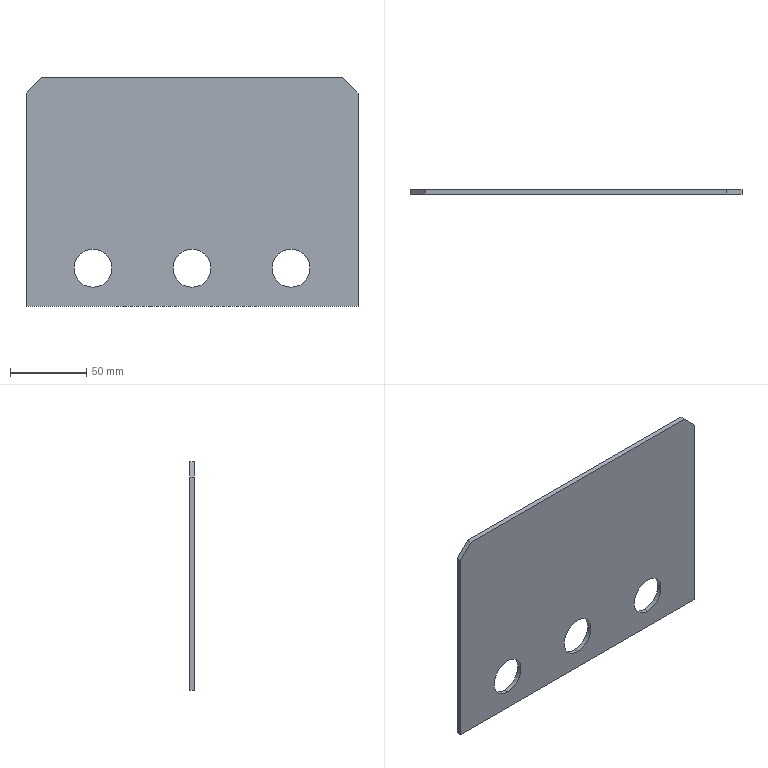Part | SolidWorks | features FlatPattern 1, SMBaseFlange 1, SheetMetal 1 | 1 solid | 14 faces | box 218 x 3 x 150 mm | volume 93382 mm3 | plane 8 | cylinder 6 | commonest cylinder face diameters 25 x6
STEP:
#1=CARTESIAN_POINT('',(65.,3.,-62.5));
#2=VERTEX_POINT('',#1);
#3=CARTESIAN_POINT('',(65.,3.,-37.5));
#4=VERTEX_POINT('',#3);
#5=CARTESIAN_POINT('',(65.,3.,-50.));
#6=DIRECTION('',(0.,1.,0.));
#7=DIRECTION('',(0.,0.,1.));
#8=AXIS2_PLACEMENT_3D('',#5,#6,#7);
#9=CIRCLE('',#8,12.5);
#10=EDGE_CURVE('',#2,#4,#9,.T.);
#11=ORIENTED_EDGE('',*,*,#10,.T.);
#12=CARTESIAN_POINT('',(65.,0.,-37.5));
#13=VERTEX_POINT('',#12);
#14=CARTESIAN_POINT('',(65.,3.,-37.5));
#15=DIRECTION('',(0.,-1.,0.));
#16=VECTOR('',#15,1000.);
#17=LINE('',#14,#16);
#18=EDGE_CURVE('',#4,#13,#17,.T.);
#19=ORIENTED_EDGE('',*,*,#18,.T.);
#20=CARTESIAN_POINT('',(65.,0.,-62.5));
#21=VERTEX_POINT('',#20);
#22=CARTESIAN_POINT('',(65.,0.,-50.));
#23=DIRECTION('',(0.,1.,0.));
#24=DIRECTION('',(0.,0.,1.));
#25=AXIS2_PLACEMENT_3D('',#22,#23,#24);
#26=CIRCLE('',#25,12.5);
#27=EDGE_CURVE('',#21,#13,#26,.T.);
#28=ORIENTED_EDGE('',*,*,#27,.F.);
#29=CARTESIAN_POINT('',(65.,3.,-62.5));
#30=DIRECTION('',(0.,-1.,0.));
#31=VECTOR('',#30,1000.);
#32=LINE('',#29,#31);
#33=EDGE_CURVE('',#2,#21,#32,.T.);
#34=ORIENTED_EDGE('',*,*,#33,.F.);
#35=EDGE_LOOP('',(#11,#19,#28,#34));
#36=FACE_OUTER_BOUND('',#35,.T.);
#37=CARTESIAN_POINT('',(65.,3.,-50.));
#38=DIRECTION('',(0.,-1.,0.));
#39=DIRECTION('',(0.,0.,-1.));
#40=AXIS2_PLACEMENT_3D('',#37,#38,#39);
#41=CYLINDRICAL_SURFACE('',#40,12.5);
#42=ADVANCED_FACE('',(#36),#41,.F.);
#43=CARTESIAN_POINT('',(0.,3.,-62.5));
#44=VERTEX_POINT('',#43);
#45=CARTESIAN_POINT('',(0.,3.,-37.5));
#46=VERTEX_POINT('',#45);
#47=CARTESIAN_POINT('',(0.,3.,-50.));
#48=DIRECTION('',(0.,1.,0.));
#49=DIRECTION('',(0.,0.,1.));
#50=AXIS2_PLACEMENT_3D('',#47,#48,#49);
#51=CIRCLE('',#50,12.5);
#52=EDGE_CURVE('',#44,#46,#51,.T.);
#53=ORIENTED_EDGE('',*,*,#52,.T.);
#54=CARTESIAN_POINT('',(0.,0.,-37.5));
#55=VERTEX_POINT('',#54);
#56=CARTESIAN_POINT('',(0.,3.,-37.5));
#57=DIRECTION('',(0.,-1.,0.));
#58=VECTOR('',#57,1000.);
#59=LINE('',#56,#58);
#60=EDGE_CURVE('',#46,#55,#59,.T.);
#61=ORIENTED_EDGE('',*,*,#60,.T.);
#62=CARTESIAN_POINT('',(0.,0.,-62.5));
#63=VERTEX_POINT('',#62);
#64=CARTESIAN_POINT('',(0.,0.,-50.));
#65=DIRECTION('',(0.,1.,0.));
#66=DIRECTION('',(0.,0.,1.));
#67=AXIS2_PLACEMENT_3D('',#64,#65,#66);
#68=CIRCLE('',#67,12.5);
#69=EDGE_CURVE('',#63,#55,#68,.T.);
#70=ORIENTED_EDGE('',*,*,#69,.F.);
#71=CARTESIAN_POINT('',(0.,3.,-62.5));
#72=DIRECTION('',(0.,-1.,0.));
#73=VECTOR('',#72,1000.);
#74=LINE('',#71,#73);
#75=EDGE_CURVE('',#44,#63,#74,.T.);
#76=ORIENTED_EDGE('',*,*,#75,.F.);
#77=EDGE_LOOP('',(#53,#61,#70,#76));
#78=FACE_OUTER_BOUND('',#77,.T.);
#79=CARTESIAN_POINT('',(0.,3.,-50.));
#80=DIRECTION('',(0.,-1.,0.));
#81=DIRECTION('',(0.,0.,-1.));
#82=AXIS2_PLACEMENT_3D('',#79,#80,#81);
#83=CYLINDRICAL_SURFACE('',#82,12.5);
#84=ADVANCED_FACE('',(#78),#83,.F.);
#85=CARTESIAN_POINT('',(-65.,3.,-62.5));
#86=VERTEX_POINT('',#85);
#87=CARTESIAN_POINT('',(-65.,3.,-37.5));
#88=VERTEX_POINT('',#87);
#89=CARTESIAN_POINT('',(-65.,3.,-50.));
#90=DIRECTION('',(0.,1.,0.));
#91=DIRECTION('',(0.,0.,1.));
#92=AXIS2_PLACEMENT_3D('',#89,#90,#91);
#93=CIRCLE('',#92,12.5);
#94=EDGE_CURVE('',#86,#88,#93,.T.);
#95=ORIENTED_EDGE('',*,*,#94,.T.);
#96=CARTESIAN_POINT('',(-65.,0.,-37.5));
#97=VERTEX_POINT('',#96);
#98=CARTESIAN_POINT('',(-65.,3.,-37.5));
#99=DIRECTION('',(0.,-1.,0.));
#100=VECTOR('',#99,1000.);
#101=LINE('',#98,#100);
#102=EDGE_CURVE('',#88,#97,#101,.T.);
#103=ORIENTED_EDGE('',*,*,#102,.T.);
#104=CARTESIAN_POINT('',(-65.,0.,-62.5));
#105=VERTEX_POINT('',#104);
#106=CARTESIAN_POINT('',(-65.,0.,-50.));
#107=DIRECTION('',(0.,1.,0.));
#108=DIRECTION('',(0.,0.,1.));
#109=AXIS2_PLACEMENT_3D('',#106,#107,#108);
#110=CIRCLE('',#109,12.5);
#111=EDGE_CURVE('',#105,#97,#110,.T.);
#112=ORIENTED_EDGE('',*,*,#111,.F.);
#113=CARTESIAN_POINT('',(-65.,3.,-62.5));
#114=DIRECTION('',(0.,-1.,0.));
#115=VECTOR('',#114,1000.);
#116=LINE('',#113,#115);
#117=EDGE_CURVE('',#86,#105,#116,.T.);
#118=ORIENTED_EDGE('',*,*,#117,.F.);
#119=EDGE_LOOP('',(#95,#103,#112,#118));
#120=FACE_OUTER_BOUND('',#119,.T.);
#121=CARTESIAN_POINT('',(-65.,3.,-50.));
#122=DIRECTION('',(0.,-1.,0.));
#123=DIRECTION('',(0.,0.,-1.));
#124=AXIS2_PLACEMENT_3D('',#121,#122,#123);
#125=CYLINDRICAL_SURFACE('',#124,12.5);
#126=ADVANCED_FACE('',(#120),#125,.F.);
#127=ORIENTED_EDGE('',*,*,#52,.F.);
#128=CARTESIAN_POINT('',(0.,3.,-50.));
#129=DIRECTION('',(0.,1.,0.));
#130=DIRECTION('',(0.,0.,1.));
#131=AXIS2_PLACEMENT_3D('',#128,#129,#130);
#132=CIRCLE('',#131,12.5);
#133=EDGE_CURVE('',#46,#44,#132,.T.);
#134=ORIENTED_EDGE('',*,*,#133,.F.);
#135=EDGE_LOOP('',(#127,#134));
#136=FACE_BOUND('',#135,.T.);
#137=CARTESIAN_POINT('',(-109.,3.,-75.));
#138=VERTEX_POINT('',#137);
#139=CARTESIAN_POINT('',(-109.,3.,65.));
#140=VERTEX_POINT('',#139);
#141=CARTESIAN_POINT('',(-109.,3.,-75.));
#142=DIRECTION('',(0.,0.,1.));
#143=VECTOR('',#142,1000.);
#144=LINE('',#141,#143);
#145=EDGE_CURVE('',#138,#140,#144,.T.);
#146=ORIENTED_EDGE('',*,*,#145,.T.);
#147=CARTESIAN_POINT('',(-99.,3.,75.));
#148=VERTEX_POINT('',#147);
#149=CARTESIAN_POINT('',(-109.,3.,65.));
#150=DIRECTION('',(0.7071,0.,0.7071));
#151=VECTOR('',#150,1000.);
#152=LINE('',#149,#151);
#153=EDGE_CURVE('',#140,#148,#152,.T.);
#154=ORIENTED_EDGE('',*,*,#153,.T.);
#155=CARTESIAN_POINT('',(99.,3.,75.));
#156=VERTEX_POINT('',#155);
#157=CARTESIAN_POINT('',(-99.,3.,75.));
#158=DIRECTION('',(1.,0.,0.));
#159=VECTOR('',#158,1000.);
#160=LINE('',#157,#159);
#161=EDGE_CURVE('',#148,#156,#160,.T.);
#162=ORIENTED_EDGE('',*,*,#161,.T.);
#163=CARTESIAN_POINT('',(109.,3.,65.));
#164=VERTEX_POINT('',#163);
#165=CARTESIAN_POINT('',(99.,3.,75.));
#166=DIRECTION('',(0.7071,0.,-0.7071));
#167=VECTOR('',#166,1000.);
#168=LINE('',#165,#167);
#169=EDGE_CURVE('',#156,#164,#168,.T.);
#170=ORIENTED_EDGE('',*,*,#169,.T.);
#171=CARTESIAN_POINT('',(109.,3.,-75.));
#172=VERTEX_POINT('',#171);
#173=CARTESIAN_POINT('',(109.,3.,-75.));
#174=DIRECTION('',(0.,0.,-1.));
#175=VECTOR('',#174,1000.);
#176=LINE('',#173,#175);
#177=EDGE_CURVE('',#164,#172,#176,.T.);
#178=ORIENTED_EDGE('',*,*,#177,.T.);
#179=CARTESIAN_POINT('',(-109.,3.,-75.));
#180=DIRECTION('',(-1.,0.,0.));
#181=VECTOR('',#180,1000.);
#182=LINE('',#179,#181);
#183=EDGE_CURVE('',#172,#138,#182,.T.);
#184=ORIENTED_EDGE('',*,*,#183,.T.);
#185=EDGE_LOOP('',(#146,#154,#162,#170,#178,#184));
#186=FACE_OUTER_BOUND('',#185,.T.);
#187=ORIENTED_EDGE('',*,*,#94,.F.);
#188=CARTESIAN_POINT('',(-65.,3.,-50.));
#189=DIRECTION('',(0.,1.,0.));
#190=DIRECTION('',(0.,0.,1.));
#191=AXIS2_PLACEMENT_3D('',#188,#189,#190);
#192=CIRCLE('',#191,12.5);
#193=EDGE_CURVE('',#88,#86,#192,.T.);
#194=ORIENTED_EDGE('',*,*,#193,.F.);
#195=EDGE_LOOP('',(#187,#194));
#196=FACE_BOUND('',#195,.T.);
#197=ORIENTED_EDGE('',*,*,#10,.F.);
#198=CARTESIAN_POINT('',(65.,3.,-50.));
#199=DIRECTION('',(0.,1.,0.));
#200=DIRECTION('',(0.,0.,1.));
#201=AXIS2_PLACEMENT_3D('',#198,#199,#200);
#202=CIRCLE('',#201,12.5);
#203=EDGE_CURVE('',#4,#2,#202,.T.);
#204=ORIENTED_EDGE('',*,*,#203,.F.);
#205=EDGE_LOOP('',(#197,#204));
#206=FACE_BOUND('',#205,.T.);
#207=CARTESIAN_POINT('',(0.,3.,0.));
#208=DIRECTION('',(0.,1.,0.));
#209=DIRECTION('',(0.,0.,1.));
#210=AXIS2_PLACEMENT_3D('',#207,#208,#209);
#211=PLANE('',#210);
#212=ADVANCED_FACE('',(#136,#186,#196,#206),#211,.T.);
#213=CARTESIAN_POINT('',(-109.,0.,-75.));
#214=VERTEX_POINT('',#213);
#215=CARTESIAN_POINT('',(-109.,0.,65.));
#216=VERTEX_POINT('',#215);
#217=CARTESIAN_POINT('',(-109.,0.,-75.));
#218=DIRECTION('',(0.,0.,1.));
#219=VECTOR('',#218,1000.);
#220=LINE('',#217,#219);
#221=EDGE_CURVE('',#214,#216,#220,.T.);
#222=ORIENTED_EDGE('',*,*,#221,.F.);
#223=CARTESIAN_POINT('',(109.,0.,-75.));
#224=VERTEX_POINT('',#223);
#225=CARTESIAN_POINT('',(-109.,0.,-75.));
#226=DIRECTION('',(-1.,0.,0.));
#227=VECTOR('',#226,1000.);
#228=LINE('',#225,#227);
#229=EDGE_CURVE('',#224,#214,#228,.T.);
#230=ORIENTED_EDGE('',*,*,#229,.F.);
#231=CARTESIAN_POINT('',(109.,0.,65.));
#232=VERTEX_POINT('',#231);
#233=CARTESIAN_POINT('',(109.,0.,-75.));
#234=DIRECTION('',(0.,0.,-1.));
#235=VECTOR('',#234,1000.);
#236=LINE('',#233,#235);
#237=EDGE_CURVE('',#232,#224,#236,.T.);
#238=ORIENTED_EDGE('',*,*,#237,.F.);
#239=CARTESIAN_POINT('',(99.,0.,75.));
#240=VERTEX_POINT('',#239);
#241=CARTESIAN_POINT('',(99.,0.,75.));
#242=DIRECTION('',(0.7071,0.,-0.7071));
#243=VECTOR('',#242,1000.);
#244=LINE('',#241,#243);
#245=EDGE_CURVE('',#240,#232,#244,.T.);
#246=ORIENTED_EDGE('',*,*,#245,.F.);
#247=CARTESIAN_POINT('',(-99.,0.,75.));
#248=VERTEX_POINT('',#247);
#249=CARTESIAN_POINT('',(-99.,0.,75.));
#250=DIRECTION('',(1.,0.,0.));
#251=VECTOR('',#250,1000.);
#252=LINE('',#249,#251);
#253=EDGE_CURVE('',#248,#240,#252,.T.);
#254=ORIENTED_EDGE('',*,*,#253,.F.);
#255=CARTESIAN_POINT('',(-109.,0.,65.));
#256=DIRECTION('',(0.7071,0.,0.7071));
#257=VECTOR('',#256,1000.);
#258=LINE('',#255,#257);
#259=EDGE_CURVE('',#216,#248,#258,.T.);
#260=ORIENTED_EDGE('',*,*,#259,.F.);
#261=EDGE_LOOP('',(#222,#230,#238,#246,#254,#260));
#262=FACE_OUTER_BOUND('',#261,.T.);
#263=ORIENTED_EDGE('',*,*,#111,.T.);
#264=CARTESIAN_POINT('',(-65.,0.,-50.));
#265=DIRECTION('',(0.,1.,0.));
#266=DIRECTION('',(0.,0.,1.));
#267=AXIS2_PLACEMENT_3D('',#264,#265,#266);
#268=CIRCLE('',#267,12.5);
#269=EDGE_CURVE('',#97,#105,#268,.T.);
#270=ORIENTED_EDGE('',*,*,#269,.T.);
#271=EDGE_LOOP('',(#263,#270));
#272=FACE_BOUND('',#271,.T.);
#273=ORIENTED_EDGE('',*,*,#69,.T.);
#274=CARTESIAN_POINT('',(0.,0.,-50.));
#275=DIRECTION('',(0.,1.,0.));
#276=DIRECTION('',(0.,0.,1.));
#277=AXIS2_PLACEMENT_3D('',#274,#275,#276);
#278=CIRCLE('',#277,12.5);
#279=EDGE_CURVE('',#55,#63,#278,.T.);
#280=ORIENTED_EDGE('',*,*,#279,.T.);
#281=EDGE_LOOP('',(#273,#280));
#282=FACE_BOUND('',#281,.T.);
#283=ORIENTED_EDGE('',*,*,#27,.T.);
#284=CARTESIAN_POINT('',(65.,0.,-50.));
#285=DIRECTION('',(0.,1.,0.));
#286=DIRECTION('',(0.,0.,1.));
#287=AXIS2_PLACEMENT_3D('',#284,#285,#286);
#288=CIRCLE('',#287,12.5);
#289=EDGE_CURVE('',#13,#21,#288,.T.);
#290=ORIENTED_EDGE('',*,*,#289,.T.);
#291=EDGE_LOOP('',(#283,#290));
#292=FACE_BOUND('',#291,.T.);
#293=CARTESIAN_POINT('',(0.,0.,0.));
#294=DIRECTION('',(0.,1.,0.));
#295=DIRECTION('',(0.,0.,1.));
#296=AXIS2_PLACEMENT_3D('',#293,#294,#295);
#297=PLANE('',#296);
#298=ADVANCED_FACE('',(#262,#272,#282,#292),#297,.F.);
#299=ORIENTED_EDGE('',*,*,#221,.T.);
#300=CARTESIAN_POINT('',(-109.,3.,65.));
#301=DIRECTION('',(0.,-1.,0.));
#302=VECTOR('',#301,1000.);
#303=LINE('',#300,#302);
#304=EDGE_CURVE('',#140,#216,#303,.T.);
#305=ORIENTED_EDGE('',*,*,#304,.F.);
#306=ORIENTED_EDGE('',*,*,#145,.F.);
#307=CARTESIAN_POINT('',(-109.,3.,-75.));
#308=DIRECTION('',(0.,-1.,0.));
#309=VECTOR('',#308,1000.);
#310=LINE('',#307,#309);
#311=EDGE_CURVE('',#138,#214,#310,.T.);
#312=ORIENTED_EDGE('',*,*,#311,.T.);
#313=EDGE_LOOP('',(#299,#305,#306,#312));
#314=FACE_OUTER_BOUND('',#313,.T.);
#315=CARTESIAN_POINT('',(-109.,3.,-75.));
#316=DIRECTION('',(1.,0.,0.));
#317=DIRECTION('',(0.,0.,-1.));
#318=AXIS2_PLACEMENT_3D('',#315,#316,#317);
#319=PLANE('',#318);
#320=ADVANCED_FACE('',(#314),#319,.F.);
#321=ORIENTED_EDGE('',*,*,#259,.T.);
#322=CARTESIAN_POINT('',(-99.,3.,75.));
#323=DIRECTION('',(0.,-1.,0.));
#324=VECTOR('',#323,1000.);
#325=LINE('',#322,#324);
#326=EDGE_CURVE('',#148,#248,#325,.T.);
#327=ORIENTED_EDGE('',*,*,#326,.F.);
#328=ORIENTED_EDGE('',*,*,#153,.F.);
#329=ORIENTED_EDGE('',*,*,#304,.T.);
#330=EDGE_LOOP('',(#321,#327,#328,#329));
#331=FACE_OUTER_BOUND('',#330,.T.);
#332=CARTESIAN_POINT('',(-109.,3.,65.));
#333=DIRECTION('',(0.7071,0.,-0.7071));
#334=DIRECTION('',(-0.7071,0.,-0.7071));
#335=AXIS2_PLACEMENT_3D('',#332,#333,#334);
#336=PLANE('',#335);
#337=ADVANCED_FACE('',(#331),#336,.F.);
#338=ORIENTED_EDGE('',*,*,#253,.T.);
#339=CARTESIAN_POINT('',(99.,3.,75.));
#340=DIRECTION('',(0.,-1.,0.));
#341=VECTOR('',#340,1000.);
#342=LINE('',#339,#341);
#343=EDGE_CURVE('',#156,#240,#342,.T.);
#344=ORIENTED_EDGE('',*,*,#343,.F.);
#345=ORIENTED_EDGE('',*,*,#161,.F.);
#346=ORIENTED_EDGE('',*,*,#326,.T.);
#347=EDGE_LOOP('',(#338,#344,#345,#346));
#348=FACE_OUTER_BOUND('',#347,.T.);
#349=CARTESIAN_POINT('',(-99.,3.,75.));
#350=DIRECTION('',(0.,0.,-1.));
#351=DIRECTION('',(-1.,0.,0.));
#352=AXIS2_PLACEMENT_3D('',#349,#350,#351);
#353=PLANE('',#352);
#354=ADVANCED_FACE('',(#348),#353,.F.);
#355=ORIENTED_EDGE('',*,*,#245,.T.);
#356=CARTESIAN_POINT('',(109.,3.,65.));
#357=DIRECTION('',(0.,-1.,0.));
#358=VECTOR('',#357,1000.);
#359=LINE('',#356,#358);
#360=EDGE_CURVE('',#164,#232,#359,.T.);
#361=ORIENTED_EDGE('',*,*,#360,.F.);
#362=ORIENTED_EDGE('',*,*,#169,.F.);
#363=ORIENTED_EDGE('',*,*,#343,.T.);
#364=EDGE_LOOP('',(#355,#361,#362,#363));
#365=FACE_OUTER_BOUND('',#364,.T.);
#366=CARTESIAN_POINT('',(99.,3.,75.));
#367=DIRECTION('',(-0.7071,0.,-0.7071));
#368=DIRECTION('',(-0.7071,0.,0.7071));
#369=AXIS2_PLACEMENT_3D('',#366,#367,#368);
#370=PLANE('',#369);
#371=ADVANCED_FACE('',(#365),#370,.F.);
#372=ORIENTED_EDGE('',*,*,#237,.T.);
#373=CARTESIAN_POINT('',(109.,3.,-75.));
#374=DIRECTION('',(0.,-1.,0.));
#375=VECTOR('',#374,1000.);
#376=LINE('',#373,#375);
#377=EDGE_CURVE('',#172,#224,#376,.T.);
#378=ORIENTED_EDGE('',*,*,#377,.F.);
#379=ORIENTED_EDGE('',*,*,#177,.F.);
#380=ORIENTED_EDGE('',*,*,#360,.T.);
#381=EDGE_LOOP('',(#372,#378,#379,#380));
#382=FACE_OUTER_BOUND('',#381,.T.);
#383=CARTESIAN_POINT('',(109.,3.,-75.));
#384=DIRECTION('',(-1.,0.,0.));
#385=DIRECTION('',(0.,0.,1.));
#386=AXIS2_PLACEMENT_3D('',#383,#384,#385);
#387=PLANE('',#386);
#388=ADVANCED_FACE('',(#382),#387,.F.);
#389=ORIENTED_EDGE('',*,*,#229,.T.);
#390=ORIENTED_EDGE('',*,*,#311,.F.);
#391=ORIENTED_EDGE('',*,*,#183,.F.);
#392=ORIENTED_EDGE('',*,*,#377,.T.);
#393=EDGE_LOOP('',(#389,#390,#391,#392));
#394=FACE_OUTER_BOUND('',#393,.T.);
#395=CARTESIAN_POINT('',(-109.,3.,-75.));
#396=DIRECTION('',(0.,0.,1.));
#397=DIRECTION('',(1.,0.,0.));
#398=AXIS2_PLACEMENT_3D('',#395,#396,#397);
#399=PLANE('',#398);
#400=ADVANCED_FACE('',(#394),#399,.F.);
#401=ORIENTED_EDGE('',*,*,#102,.F.);
#402=ORIENTED_EDGE('',*,*,#193,.T.);
#403=ORIENTED_EDGE('',*,*,#117,.T.);
#404=ORIENTED_EDGE('',*,*,#269,.F.);
#405=EDGE_LOOP('',(#401,#402,#403,#404));
#406=FACE_OUTER_BOUND('',#405,.T.);
#407=CARTESIAN_POINT('',(-65.,3.,-50.));
#408=DIRECTION('',(0.,-1.,0.));
#409=DIRECTION('',(0.,0.,-1.));
#410=AXIS2_PLACEMENT_3D('',#407,#408,#409);
#411=CYLINDRICAL_SURFACE('',#410,12.5);
#412=ADVANCED_FACE('',(#406),#411,.F.);
#413=ORIENTED_EDGE('',*,*,#60,.F.);
#414=ORIENTED_EDGE('',*,*,#133,.T.);
#415=ORIENTED_EDGE('',*,*,#75,.T.);
#416=ORIENTED_EDGE('',*,*,#279,.F.);
#417=EDGE_LOOP('',(#413,#414,#415,#416));
#418=FACE_OUTER_BOUND('',#417,.T.);
#419=CARTESIAN_POINT('',(0.,3.,-50.));
#420=DIRECTION('',(0.,-1.,0.));
#421=DIRECTION('',(0.,0.,-1.));
#422=AXIS2_PLACEMENT_3D('',#419,#420,#421);
#423=CYLINDRICAL_SURFACE('',#422,12.5);
#424=ADVANCED_FACE('',(#418),#423,.F.);
#425=ORIENTED_EDGE('',*,*,#18,.F.);
#426=ORIENTED_EDGE('',*,*,#203,.T.);
#427=ORIENTED_EDGE('',*,*,#33,.T.);
#428=ORIENTED_EDGE('',*,*,#289,.F.);
#429=EDGE_LOOP('',(#425,#426,#427,#428));
#430=FACE_OUTER_BOUND('',#429,.T.);
#431=CARTESIAN_POINT('',(65.,3.,-50.));
#432=DIRECTION('',(0.,-1.,0.));
#433=DIRECTION('',(0.,0.,-1.));
#434=AXIS2_PLACEMENT_3D('',#431,#432,#433);
#435=CYLINDRICAL_SURFACE('',#434,12.5);
#436=ADVANCED_FACE('',(#430),#435,.F.);
#437=CLOSED_SHELL('',(#42,#84,#126,#212,#298,#320,#337,#354,#371,#388,#400,#412,#424,#436));
#438=MANIFOLD_SOLID_BREP('',#437);
#439=CARTESIAN_POINT('',(0.,0.,0.));
#440=DIRECTION('',(0.,0.,1.));
#441=DIRECTION('',(1.,0.,0.));
#442=AXIS2_PLACEMENT_3D('',#439,#440,#441);
#443=(LENGTH_UNIT()NAMED_UNIT(*)SI_UNIT(.MILLI.,.METRE.));
#444=UNCERTAINTY_MEASURE_WITH_UNIT(LENGTH_MEASURE(0.00001),#443,'','');
#445=(NAMED_UNIT(*)PLANE_ANGLE_UNIT()SI_UNIT($,.RADIAN.));
#446=(NAMED_UNIT(*)SI_UNIT($,.STERADIAN.)SOLID_ANGLE_UNIT());
#447=(GEOMETRIC_REPRESENTATION_CONTEXT(3)GLOBAL_UNCERTAINTY_ASSIGNED_CONTEXT((#444))GLOBAL_UNIT_ASSIGNED_CONTEXT((#443,#445,#446))REPRESENTATION_CONTEXT('',''));
#448=ADVANCED_BREP_SHAPE_REPRESENTATION('',(#438,#442),#447);